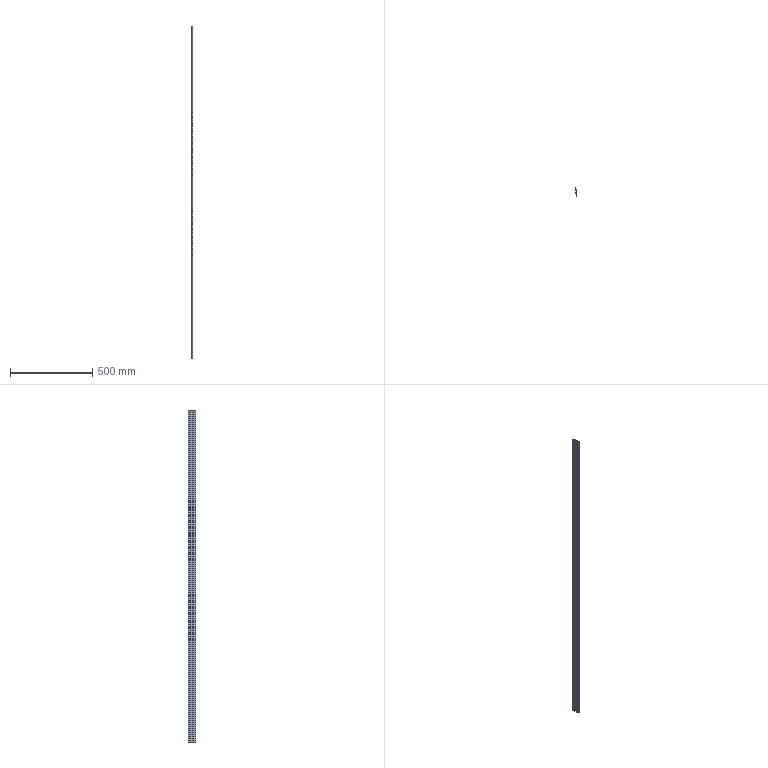Part | 1 solid | 33 faces | box 9.4 x 46.998 x 2016 mm | volume 227729 mm3 | plane 22 | cylinder 11 | commonest cylinder face diameters 0.24 x2 0.4 x2 0.8 x2 1.2 x2 6 x2 1 x1
STEP:
#1=CARTESIAN_POINT('',(-2.9,32.45,-1008.));
#2=VERTEX_POINT('',#1);
#3=CARTESIAN_POINT('',(-2.7,32.25,-1008.));
#4=VERTEX_POINT('',#3);
#5=CARTESIAN_POINT('',(-2.7,32.45,-1008.));
#6=DIRECTION('',(0.,0.,1.));
#7=DIRECTION('',(1.,0.,0.));
#8=AXIS2_PLACEMENT_3D('',#5,#6,#7);
#9=CIRCLE('',#8,0.2);
#10=EDGE_CURVE('',#2,#4,#9,.T.);
#11=ORIENTED_EDGE('',*,*,#10,.T.);
#12=CARTESIAN_POINT('',(-2.7,32.25,1008.));
#13=VERTEX_POINT('',#12);
#14=CARTESIAN_POINT('',(-2.7,32.25,1008.));
#15=DIRECTION('',(0.,0.,-1.));
#16=VECTOR('',#15,1000.);
#17=LINE('',#14,#16);
#18=EDGE_CURVE('',#13,#4,#17,.T.);
#19=ORIENTED_EDGE('',*,*,#18,.F.);
#20=CARTESIAN_POINT('',(-2.9,32.45,1008.));
#21=VERTEX_POINT('',#20);
#22=CARTESIAN_POINT('',(-2.7,32.45,1008.));
#23=DIRECTION('',(0.,0.,1.));
#24=DIRECTION('',(1.,0.,0.));
#25=AXIS2_PLACEMENT_3D('',#22,#23,#24);
#26=CIRCLE('',#25,0.2);
#27=EDGE_CURVE('',#21,#13,#26,.T.);
#28=ORIENTED_EDGE('',*,*,#27,.F.);
#29=CARTESIAN_POINT('',(-2.9,32.45,1008.));
#30=DIRECTION('',(0.,0.,-1.));
#31=VECTOR('',#30,1000.);
#32=LINE('',#29,#31);
#33=EDGE_CURVE('',#21,#2,#32,.T.);
#34=ORIENTED_EDGE('',*,*,#33,.T.);
#35=EDGE_LOOP('',(#11,#19,#28,#34));
#36=FACE_OUTER_BOUND('',#35,.T.);
#37=CARTESIAN_POINT('',(-2.7,32.45,1008.));
#38=DIRECTION('',(0.,0.,-1.));
#39=DIRECTION('',(-1.,0.,0.));
#40=AXIS2_PLACEMENT_3D('',#37,#38,#39);
#41=CYLINDRICAL_SURFACE('',#40,0.2);
#42=ADVANCED_FACE('',(#36),#41,.T.);
#43=CARTESIAN_POINT('',(-2.5,32.25,-1008.));
#44=VERTEX_POINT('',#43);
#45=CARTESIAN_POINT('',(-2.7,32.25,-1008.));
#46=DIRECTION('',(1.,0.,0.));
#47=VECTOR('',#46,1000.);
#48=LINE('',#45,#47);
#49=EDGE_CURVE('',#4,#44,#48,.T.);
#50=ORIENTED_EDGE('',*,*,#49,.T.);
#51=CARTESIAN_POINT('',(-2.5,32.25,1008.));
#52=VERTEX_POINT('',#51);
#53=CARTESIAN_POINT('',(-2.5,32.25,1008.));
#54=DIRECTION('',(0.,0.,-1.));
#55=VECTOR('',#54,1000.);
#56=LINE('',#53,#55);
#57=EDGE_CURVE('',#52,#44,#56,.T.);
#58=ORIENTED_EDGE('',*,*,#57,.F.);
#59=CARTESIAN_POINT('',(-2.7,32.25,1008.));
#60=DIRECTION('',(1.,0.,0.));
#61=VECTOR('',#60,1000.);
#62=LINE('',#59,#61);
#63=EDGE_CURVE('',#13,#52,#62,.T.);
#64=ORIENTED_EDGE('',*,*,#63,.F.);
#65=ORIENTED_EDGE('',*,*,#18,.T.);
#66=EDGE_LOOP('',(#50,#58,#64,#65));
#67=FACE_OUTER_BOUND('',#66,.T.);
#68=CARTESIAN_POINT('',(-2.7,32.25,1008.));
#69=DIRECTION('',(0.,1.,0.));
#70=DIRECTION('',(0.,0.,1.));
#71=AXIS2_PLACEMENT_3D('',#68,#69,#70);
#72=PLANE('',#71);
#73=ADVANCED_FACE('',(#67),#72,.F.);
#74=CARTESIAN_POINT('',(-1.9,32.85,-1008.));
#75=VERTEX_POINT('',#74);
#76=CARTESIAN_POINT('',(-2.5,32.85,-1008.));
#77=DIRECTION('',(0.,0.,1.));
#78=DIRECTION('',(1.,0.,0.));
#79=AXIS2_PLACEMENT_3D('',#76,#77,#78);
#80=CIRCLE('',#79,0.6);
#81=EDGE_CURVE('',#44,#75,#80,.T.);
#82=ORIENTED_EDGE('',*,*,#81,.T.);
#83=CARTESIAN_POINT('',(-1.9,32.85,1008.));
#84=VERTEX_POINT('',#83);
#85=CARTESIAN_POINT('',(-1.9,32.85,1008.));
#86=DIRECTION('',(0.,0.,-1.));
#87=VECTOR('',#86,1000.);
#88=LINE('',#85,#87);
#89=EDGE_CURVE('',#84,#75,#88,.T.);
#90=ORIENTED_EDGE('',*,*,#89,.F.);
#91=CARTESIAN_POINT('',(-2.5,32.85,1008.));
#92=DIRECTION('',(0.,0.,1.));
#93=DIRECTION('',(1.,0.,0.));
#94=AXIS2_PLACEMENT_3D('',#91,#92,#93);
#95=CIRCLE('',#94,0.6);
#96=EDGE_CURVE('',#52,#84,#95,.T.);
#97=ORIENTED_EDGE('',*,*,#96,.F.);
#98=ORIENTED_EDGE('',*,*,#57,.T.);
#99=EDGE_LOOP('',(#82,#90,#97,#98));
#100=FACE_OUTER_BOUND('',#99,.T.);
#101=CARTESIAN_POINT('',(-2.5,32.85,1008.));
#102=DIRECTION('',(0.,0.,-1.));
#103=DIRECTION('',(-1.,0.,0.));
#104=AXIS2_PLACEMENT_3D('',#101,#102,#103);
#105=CYLINDRICAL_SURFACE('',#104,0.6);
#106=ADVANCED_FACE('',(#100),#105,.T.);
#107=CARTESIAN_POINT('',(-1.9,36.13,-1008.));
#108=VERTEX_POINT('',#107);
#109=CARTESIAN_POINT('',(-1.9,32.85,-1008.));
#110=DIRECTION('',(0.,1.,0.));
#111=VECTOR('',#110,1000.);
#112=LINE('',#109,#111);
#113=EDGE_CURVE('',#75,#108,#112,.T.);
#114=ORIENTED_EDGE('',*,*,#113,.T.);
#115=CARTESIAN_POINT('',(-1.9,36.13,1008.));
#116=VERTEX_POINT('',#115);
#117=CARTESIAN_POINT('',(-1.9,36.13,1008.));
#118=DIRECTION('',(0.,0.,-1.));
#119=VECTOR('',#118,1000.);
#120=LINE('',#117,#119);
#121=EDGE_CURVE('',#116,#108,#120,.T.);
#122=ORIENTED_EDGE('',*,*,#121,.F.);
#123=CARTESIAN_POINT('',(-1.9,32.85,1008.));
#124=DIRECTION('',(0.,1.,0.));
#125=VECTOR('',#124,1000.);
#126=LINE('',#123,#125);
#127=EDGE_CURVE('',#84,#116,#126,.T.);
#128=ORIENTED_EDGE('',*,*,#127,.F.);
#129=ORIENTED_EDGE('',*,*,#89,.T.);
#130=EDGE_LOOP('',(#114,#122,#128,#129));
#131=FACE_OUTER_BOUND('',#130,.T.);
#132=CARTESIAN_POINT('',(-1.9,32.85,1008.));
#133=DIRECTION('',(-1.,0.,0.));
#134=DIRECTION('',(0.,0.,1.));
#135=AXIS2_PLACEMENT_3D('',#132,#133,#134);
#136=PLANE('',#135);
#137=ADVANCED_FACE('',(#131),#136,.F.);
#138=CARTESIAN_POINT('',(-1.78,36.25,-1008.));
#139=VERTEX_POINT('',#138);
#140=CARTESIAN_POINT('',(-1.78,36.13,-1008.));
#141=DIRECTION('',(0.,0.,-1.));
#142=DIRECTION('',(1.,0.,0.));
#143=AXIS2_PLACEMENT_3D('',#140,#141,#142);
#144=CIRCLE('',#143,0.12);
#145=EDGE_CURVE('',#108,#139,#144,.T.);
#146=ORIENTED_EDGE('',*,*,#145,.T.);
#147=CARTESIAN_POINT('',(-1.78,36.25,1008.));
#148=VERTEX_POINT('',#147);
#149=CARTESIAN_POINT('',(-1.78,36.25,1008.));
#150=DIRECTION('',(0.,0.,-1.));
#151=VECTOR('',#150,1000.);
#152=LINE('',#149,#151);
#153=EDGE_CURVE('',#148,#139,#152,.T.);
#154=ORIENTED_EDGE('',*,*,#153,.F.);
#155=CARTESIAN_POINT('',(-1.78,36.13,1008.));
#156=DIRECTION('',(0.,0.,-1.));
#157=DIRECTION('',(1.,0.,0.));
#158=AXIS2_PLACEMENT_3D('',#155,#156,#157);
#159=CIRCLE('',#158,0.12);
#160=EDGE_CURVE('',#116,#148,#159,.T.);
#161=ORIENTED_EDGE('',*,*,#160,.F.);
#162=ORIENTED_EDGE('',*,*,#121,.T.);
#163=EDGE_LOOP('',(#146,#154,#161,#162));
#164=FACE_OUTER_BOUND('',#163,.T.);
#165=CARTESIAN_POINT('',(-1.78,36.13,1008.));
#166=DIRECTION('',(0.,0.,-1.));
#167=DIRECTION('',(-1.,0.,0.));
#168=AXIS2_PLACEMENT_3D('',#165,#166,#167);
#169=CYLINDRICAL_SURFACE('',#168,0.12);
#170=ADVANCED_FACE('',(#164),#169,.F.);
#171=CARTESIAN_POINT('',(0.,36.25,-1008.));
#172=VERTEX_POINT('',#171);
#173=CARTESIAN_POINT('',(-1.78,36.25,-1008.));
#174=DIRECTION('',(1.,0.,0.));
#175=VECTOR('',#174,1000.);
#176=LINE('',#173,#175);
#177=EDGE_CURVE('',#139,#172,#176,.T.);
#178=ORIENTED_EDGE('',*,*,#177,.T.);
#179=CARTESIAN_POINT('',(0.,36.25,1008.));
#180=VERTEX_POINT('',#179);
#181=CARTESIAN_POINT('',(0.,36.25,1008.));
#182=DIRECTION('',(0.,0.,-1.));
#183=VECTOR('',#182,1000.);
#184=LINE('',#181,#183);
#185=EDGE_CURVE('',#180,#172,#184,.T.);
#186=ORIENTED_EDGE('',*,*,#185,.F.);
#187=CARTESIAN_POINT('',(-1.78,36.25,1008.));
#188=DIRECTION('',(1.,0.,0.));
#189=VECTOR('',#188,1000.);
#190=LINE('',#187,#189);
#191=EDGE_CURVE('',#148,#180,#190,.T.);
#192=ORIENTED_EDGE('',*,*,#191,.F.);
#193=ORIENTED_EDGE('',*,*,#153,.T.);
#194=EDGE_LOOP('',(#178,#186,#192,#193));
#195=FACE_OUTER_BOUND('',#194,.T.);
#196=CARTESIAN_POINT('',(-1.78,36.25,1008.));
#197=DIRECTION('',(0.,1.,0.));
#198=DIRECTION('',(0.,0.,1.));
#199=AXIS2_PLACEMENT_3D('',#196,#197,#198);
#200=PLANE('',#199);
#201=ADVANCED_FACE('',(#195),#200,.F.);
#202=CARTESIAN_POINT('',(0.0007641,20.449,-1008.));
#203=VERTEX_POINT('',#202);
#204=CARTESIAN_POINT('',(0.,36.25,-1008.));
#205=DIRECTION('',(0.00004836,-1.,0.));
#206=VECTOR('',#205,1000.);
#207=LINE('',#204,#206);
#208=EDGE_CURVE('',#172,#203,#207,.T.);
#209=ORIENTED_EDGE('',*,*,#208,.T.);
#210=CARTESIAN_POINT('',(0.0007641,20.449,1008.));
#211=VERTEX_POINT('',#210);
#212=CARTESIAN_POINT('',(0.0007641,20.449,1008.));
#213=DIRECTION('',(0.,0.,-1.));
#214=VECTOR('',#213,1000.);
#215=LINE('',#212,#214);
#216=EDGE_CURVE('',#211,#203,#215,.T.);
#217=ORIENTED_EDGE('',*,*,#216,.F.);
#218=CARTESIAN_POINT('',(0.,36.25,1008.));
#219=DIRECTION('',(0.00004836,-1.,0.));
#220=VECTOR('',#219,1000.);
#221=LINE('',#218,#220);
#222=EDGE_CURVE('',#180,#211,#221,.T.);
#223=ORIENTED_EDGE('',*,*,#222,.F.);
#224=ORIENTED_EDGE('',*,*,#185,.T.);
#225=EDGE_LOOP('',(#209,#217,#223,#224));
#226=FACE_OUTER_BOUND('',#225,.T.);
#227=CARTESIAN_POINT('',(0.,36.25,1008.));
#228=DIRECTION('',(1.,0.00004836,0.));
#229=DIRECTION('',(-0.00004836,1.,0.));
#230=AXIS2_PLACEMENT_3D('',#227,#228,#229);
#231=PLANE('',#230);
#232=ADVANCED_FACE('',(#226),#231,.F.);
#233=CARTESIAN_POINT('',(-2.499,20.449,-1008.));
#234=VERTEX_POINT('',#233);
#235=CARTESIAN_POINT('',(0.0007641,20.449,-1008.));
#236=DIRECTION('',(-1.,0.,0.));
#237=VECTOR('',#236,1000.);
#238=LINE('',#235,#237);
#239=EDGE_CURVE('',#203,#234,#238,.T.);
#240=ORIENTED_EDGE('',*,*,#239,.T.);
#241=CARTESIAN_POINT('',(-2.499,20.449,1008.));
#242=VERTEX_POINT('',#241);
#243=CARTESIAN_POINT('',(-2.499,20.449,1008.));
#244=DIRECTION('',(0.,0.,-1.));
#245=VECTOR('',#244,1000.);
#246=LINE('',#243,#245);
#247=EDGE_CURVE('',#242,#234,#246,.T.);
#248=ORIENTED_EDGE('',*,*,#247,.F.);
#249=CARTESIAN_POINT('',(0.0007641,20.449,1008.));
#250=DIRECTION('',(-1.,0.,0.));
#251=VECTOR('',#250,1000.);
#252=LINE('',#249,#251);
#253=EDGE_CURVE('',#211,#242,#252,.T.);
#254=ORIENTED_EDGE('',*,*,#253,.F.);
#255=ORIENTED_EDGE('',*,*,#216,.T.);
#256=EDGE_LOOP('',(#240,#248,#254,#255));
#257=FACE_OUTER_BOUND('',#256,.T.);
#258=CARTESIAN_POINT('',(0.0007641,20.449,1008.));
#259=DIRECTION('',(0.,-1.,0.));
#260=DIRECTION('',(0.,0.,-1.));
#261=AXIS2_PLACEMENT_3D('',#258,#259,#260);
#262=PLANE('',#261);
#263=ADVANCED_FACE('',(#257),#262,.F.);
#264=CARTESIAN_POINT('',(-2.899,20.049,-1008.));
#265=VERTEX_POINT('',#264);
#266=CARTESIAN_POINT('',(-2.499,20.049,-1008.));
#267=DIRECTION('',(0.,0.,1.));
#268=DIRECTION('',(1.,0.,0.));
#269=AXIS2_PLACEMENT_3D('',#266,#267,#268);
#270=CIRCLE('',#269,0.4);
#271=EDGE_CURVE('',#234,#265,#270,.T.);
#272=ORIENTED_EDGE('',*,*,#271,.T.);
#273=CARTESIAN_POINT('',(-2.899,20.049,1008.));
#274=VERTEX_POINT('',#273);
#275=CARTESIAN_POINT('',(-2.899,20.049,1008.));
#276=DIRECTION('',(0.,0.,-1.));
#277=VECTOR('',#276,1000.);
#278=LINE('',#275,#277);
#279=EDGE_CURVE('',#274,#265,#278,.T.);
#280=ORIENTED_EDGE('',*,*,#279,.F.);
#281=CARTESIAN_POINT('',(-2.499,20.049,1008.));
#282=DIRECTION('',(0.,0.,1.));
#283=DIRECTION('',(1.,0.,0.));
#284=AXIS2_PLACEMENT_3D('',#281,#282,#283);
#285=CIRCLE('',#284,0.4);
#286=EDGE_CURVE('',#242,#274,#285,.T.);
#287=ORIENTED_EDGE('',*,*,#286,.F.);
#288=ORIENTED_EDGE('',*,*,#247,.T.);
#289=EDGE_LOOP('',(#272,#280,#287,#288));
#290=FACE_OUTER_BOUND('',#289,.T.);
#291=CARTESIAN_POINT('',(-2.499,20.049,1008.));
#292=DIRECTION('',(0.,0.,-1.));
#293=DIRECTION('',(-1.,0.,0.));
#294=AXIS2_PLACEMENT_3D('',#291,#292,#293);
#295=CYLINDRICAL_SURFACE('',#294,0.4);
#296=ADVANCED_FACE('',(#290),#295,.T.);
#297=CARTESIAN_POINT('',(-2.899,15.65,-1008.));
#298=VERTEX_POINT('',#297);
#299=CARTESIAN_POINT('',(-2.899,20.049,-1008.));
#300=DIRECTION('',(0.,-1.,0.));
#301=VECTOR('',#300,1000.);
#302=LINE('',#299,#301);
#303=EDGE_CURVE('',#265,#298,#302,.T.);
#304=ORIENTED_EDGE('',*,*,#303,.T.);
#305=CARTESIAN_POINT('',(-2.899,15.65,1008.));
#306=VERTEX_POINT('',#305);
#307=CARTESIAN_POINT('',(-2.899,15.65,1008.));
#308=DIRECTION('',(0.,0.,-1.));
#309=VECTOR('',#308,1000.);
#310=LINE('',#307,#309);
#311=EDGE_CURVE('',#306,#298,#310,.T.);
#312=ORIENTED_EDGE('',*,*,#311,.F.);
#313=CARTESIAN_POINT('',(-2.899,20.049,1008.));
#314=DIRECTION('',(0.,-1.,0.));
#315=VECTOR('',#314,1000.);
#316=LINE('',#313,#315);
#317=EDGE_CURVE('',#274,#306,#316,.T.);
#318=ORIENTED_EDGE('',*,*,#317,.F.);
#319=ORIENTED_EDGE('',*,*,#279,.T.);
#320=EDGE_LOOP('',(#304,#312,#318,#319));
#321=FACE_OUTER_BOUND('',#320,.T.);
#322=CARTESIAN_POINT('',(-2.899,20.049,1008.));
#323=DIRECTION('',(1.,0.,0.));
#324=DIRECTION('',(0.,0.,-1.));
#325=AXIS2_PLACEMENT_3D('',#322,#323,#324);
#326=PLANE('',#325);
#327=ADVANCED_FACE('',(#321),#326,.F.);
#328=CARTESIAN_POINT('',(-2.699,15.45,-1008.));
#329=VERTEX_POINT('',#328);
#330=CARTESIAN_POINT('',(-2.699,15.65,-1008.));
#331=DIRECTION('',(0.,0.,1.));
#332=DIRECTION('',(1.,0.,0.));
#333=AXIS2_PLACEMENT_3D('',#330,#331,#332);
#334=CIRCLE('',#333,0.2);
#335=EDGE_CURVE('',#298,#329,#334,.T.);
#336=ORIENTED_EDGE('',*,*,#335,.T.);
#337=CARTESIAN_POINT('',(-2.699,15.45,1008.));
#338=VERTEX_POINT('',#337);
#339=CARTESIAN_POINT('',(-2.699,15.45,1008.));
#340=DIRECTION('',(0.,0.,-1.));
#341=VECTOR('',#340,1000.);
#342=LINE('',#339,#341);
#343=EDGE_CURVE('',#338,#329,#342,.T.);
#344=ORIENTED_EDGE('',*,*,#343,.F.);
#345=CARTESIAN_POINT('',(-2.699,15.65,1008.));
#346=DIRECTION('',(0.,0.,1.));
#347=DIRECTION('',(1.,0.,0.));
#348=AXIS2_PLACEMENT_3D('',#345,#346,#347);
#349=CIRCLE('',#348,0.2);
#350=EDGE_CURVE('',#306,#338,#349,.T.);
#351=ORIENTED_EDGE('',*,*,#350,.F.);
#352=ORIENTED_EDGE('',*,*,#311,.T.);
#353=EDGE_LOOP('',(#336,#344,#351,#352));
#354=FACE_OUTER_BOUND('',#353,.T.);
#355=CARTESIAN_POINT('',(-2.699,15.65,1008.));
#356=DIRECTION('',(0.,0.,-1.));
#357=DIRECTION('',(-1.,0.,0.));
#358=AXIS2_PLACEMENT_3D('',#355,#356,#357);
#359=CYLINDRICAL_SURFACE('',#358,0.2);
#360=ADVANCED_FACE('',(#354),#359,.T.);
#361=CARTESIAN_POINT('',(-2.499,15.45,-1008.));
#362=VERTEX_POINT('',#361);
#363=CARTESIAN_POINT('',(-2.699,15.45,-1008.));
#364=DIRECTION('',(1.,0.,0.));
#365=VECTOR('',#364,1000.);
#366=LINE('',#363,#365);
#367=EDGE_CURVE('',#329,#362,#366,.T.);
#368=ORIENTED_EDGE('',*,*,#367,.T.);
#369=CARTESIAN_POINT('',(-2.499,15.45,1008.));
#370=VERTEX_POINT('',#369);
#371=CARTESIAN_POINT('',(-2.499,15.45,1008.));
#372=DIRECTION('',(0.,0.,-1.));
#373=VECTOR('',#372,1000.);
#374=LINE('',#371,#373);
#375=EDGE_CURVE('',#370,#362,#374,.T.);
#376=ORIENTED_EDGE('',*,*,#375,.F.);
#377=CARTESIAN_POINT('',(-2.699,15.45,1008.));
#378=DIRECTION('',(1.,0.,0.));
#379=VECTOR('',#378,1000.);
#380=LINE('',#377,#379);
#381=EDGE_CURVE('',#338,#370,#380,.T.);
#382=ORIENTED_EDGE('',*,*,#381,.F.);
#383=ORIENTED_EDGE('',*,*,#343,.T.);
#384=EDGE_LOOP('',(#368,#376,#382,#383));
#385=FACE_OUTER_BOUND('',#384,.T.);
#386=CARTESIAN_POINT('',(-2.699,15.45,1008.));
#387=DIRECTION('',(0.,1.,0.));
#388=DIRECTION('',(0.,0.,1.));
#389=AXIS2_PLACEMENT_3D('',#386,#387,#388);
#390=PLANE('',#389);
#391=ADVANCED_FACE('',(#385),#390,.F.);
#392=CARTESIAN_POINT('',(-1.899,16.05,-1008.));
#393=VERTEX_POINT('',#392);
#394=CARTESIAN_POINT('',(-2.499,16.05,-1008.));
#395=DIRECTION('',(0.,0.,1.));
#396=DIRECTION('',(1.,0.,0.));
#397=AXIS2_PLACEMENT_3D('',#394,#395,#396);
#398=CIRCLE('',#397,0.6);
#399=EDGE_CURVE('',#362,#393,#398,.T.);
#400=ORIENTED_EDGE('',*,*,#399,.T.);
#401=CARTESIAN_POINT('',(-1.899,16.05,1008.));
#402=VERTEX_POINT('',#401);
#403=CARTESIAN_POINT('',(-1.899,16.05,1008.));
#404=DIRECTION('',(0.,0.,-1.));
#405=VECTOR('',#404,1000.);
#406=LINE('',#403,#405);
#407=EDGE_CURVE('',#402,#393,#406,.T.);
#408=ORIENTED_EDGE('',*,*,#407,.F.);
#409=CARTESIAN_POINT('',(-2.499,16.05,1008.));
#410=DIRECTION('',(0.,0.,1.));
#411=DIRECTION('',(1.,0.,0.));
#412=AXIS2_PLACEMENT_3D('',#409,#410,#411);
#413=CIRCLE('',#412,0.6);
#414=EDGE_CURVE('',#370,#402,#413,.T.);
#415=ORIENTED_EDGE('',*,*,#414,.F.);
#416=ORIENTED_EDGE('',*,*,#375,.T.);
#417=EDGE_LOOP('',(#400,#408,#415,#416));
#418=FACE_OUTER_BOUND('',#417,.T.);
#419=CARTESIAN_POINT('',(-2.499,16.05,1008.));
#420=DIRECTION('',(0.,0.,-1.));
#421=DIRECTION('',(-1.,0.,0.));
#422=AXIS2_PLACEMENT_3D('',#419,#420,#421);
#423=CYLINDRICAL_SURFACE('',#422,0.6);
#424=ADVANCED_FACE('',(#418),#423,.T.);
#425=CARTESIAN_POINT('',(-1.899,19.329,-1008.));
#426=VERTEX_POINT('',#425);
#427=CARTESIAN_POINT('',(-1.899,16.05,-1008.));
#428=DIRECTION('',(0.,1.,0.));
#429=VECTOR('',#428,1000.);
#430=LINE('',#427,#429);
#431=EDGE_CURVE('',#393,#426,#430,.T.);
#432=ORIENTED_EDGE('',*,*,#431,.T.);
#433=CARTESIAN_POINT('',(-1.899,19.329,1008.));
#434=VERTEX_POINT('',#433);
#435=CARTESIAN_POINT('',(-1.899,19.329,1008.));
#436=DIRECTION('',(0.,0.,-1.));
#437=VECTOR('',#436,1000.);
#438=LINE('',#435,#437);
#439=EDGE_CURVE('',#434,#426,#438,.T.);
#440=ORIENTED_EDGE('',*,*,#439,.F.);
#441=CARTESIAN_POINT('',(-1.899,16.05,1008.));
#442=DIRECTION('',(0.,1.,0.));
#443=VECTOR('',#442,1000.);
#444=LINE('',#441,#443);
#445=EDGE_CURVE('',#402,#434,#444,.T.);
#446=ORIENTED_EDGE('',*,*,#445,.F.);
#447=ORIENTED_EDGE('',*,*,#407,.T.);
#448=EDGE_LOOP('',(#432,#440,#446,#447));
#449=FACE_OUTER_BOUND('',#448,.T.);
#450=CARTESIAN_POINT('',(-1.899,16.05,1008.));
#451=DIRECTION('',(-1.,0.,0.));
#452=DIRECTION('',(0.,0.,1.));
#453=AXIS2_PLACEMENT_3D('',#450,#451,#452);
#454=PLANE('',#453);
#455=ADVANCED_FACE('',(#449),#454,.F.);
#456=CARTESIAN_POINT('',(-1.779,19.449,-1008.));
#457=VERTEX_POINT('',#456);
#458=CARTESIAN_POINT('',(-1.779,19.329,-1008.));
#459=DIRECTION('',(0.,0.,-1.));
#460=DIRECTION('',(1.,0.,0.));
#461=AXIS2_PLACEMENT_3D('',#458,#459,#460);
#462=CIRCLE('',#461,0.12);
#463=EDGE_CURVE('',#426,#457,#462,.T.);
#464=ORIENTED_EDGE('',*,*,#463,.T.);
#465=CARTESIAN_POINT('',(-1.779,19.449,1008.));
#466=VERTEX_POINT('',#465);
#467=CARTESIAN_POINT('',(-1.779,19.449,1008.));
#468=DIRECTION('',(0.,0.,-1.));
#469=VECTOR('',#468,1000.);
#470=LINE('',#467,#469);
#471=EDGE_CURVE('',#466,#457,#470,.T.);
#472=ORIENTED_EDGE('',*,*,#471,.F.);
#473=CARTESIAN_POINT('',(-1.779,19.329,1008.));
#474=DIRECTION('',(0.,0.,-1.));
#475=DIRECTION('',(1.,0.,0.));
#476=AXIS2_PLACEMENT_3D('',#473,#474,#475);
#477=CIRCLE('',#476,0.12);
#478=EDGE_CURVE('',#434,#466,#477,.T.);
#479=ORIENTED_EDGE('',*,*,#478,.F.);
#480=ORIENTED_EDGE('',*,*,#439,.T.);
#481=EDGE_LOOP('',(#464,#472,#479,#480));
#482=FACE_OUTER_BOUND('',#481,.T.);
#483=CARTESIAN_POINT('',(-1.779,19.329,1008.));
#484=DIRECTION('',(0.,0.,-1.));
#485=DIRECTION('',(-1.,0.,0.));
#486=AXIS2_PLACEMENT_3D('',#483,#484,#485);
#487=CYLINDRICAL_SURFACE('',#486,0.12);
#488=ADVANCED_FACE('',(#482),#487,.F.);
#489=CARTESIAN_POINT('',(0.0007641,19.449,-1008.));
#490=VERTEX_POINT('',#489);
#491=CARTESIAN_POINT('',(-1.779,19.449,-1008.));
#492=DIRECTION('',(1.,0.,0.));
#493=VECTOR('',#492,1000.);
#494=LINE('',#491,#493);
#495=EDGE_CURVE('',#457,#490,#494,.T.);
#496=ORIENTED_EDGE('',*,*,#495,.T.);
#497=CARTESIAN_POINT('',(0.0007641,19.449,1008.));
#498=VERTEX_POINT('',#497);
#499=CARTESIAN_POINT('',(0.0007641,19.449,1008.));
#500=DIRECTION('',(0.,0.,-1.));
#501=VECTOR('',#500,1000.);
#502=LINE('',#499,#501);
#503=EDGE_CURVE('',#498,#490,#502,.T.);
#504=ORIENTED_EDGE('',*,*,#503,.F.);
#505=CARTESIAN_POINT('',(-1.779,19.449,1008.));
#506=DIRECTION('',(1.,0.,0.));
#507=VECTOR('',#506,1000.);
#508=LINE('',#505,#507);
#509=EDGE_CURVE('',#466,#498,#508,.T.);
#510=ORIENTED_EDGE('',*,*,#509,.F.);
#511=ORIENTED_EDGE('',*,*,#471,.T.);
#512=EDGE_LOOP('',(#496,#504,#510,#511));
#513=FACE_OUTER_BOUND('',#512,.T.);
#514=CARTESIAN_POINT('',(-1.779,19.449,1008.));
#515=DIRECTION('',(0.,1.,0.));
#516=DIRECTION('',(0.,0.,1.));
#517=AXIS2_PLACEMENT_3D('',#514,#515,#516);
#518=PLANE('',#517);
#519=ADVANCED_FACE('',(#513),#518,.F.);
#520=CARTESIAN_POINT('',(0.,0.,-1008.));
#521=VERTEX_POINT('',#520);
#522=CARTESIAN_POINT('',(0.0007641,19.449,-1008.));
#523=DIRECTION('',(-0.00003929,-1.,0.));
#524=VECTOR('',#523,1000.);
#525=LINE('',#522,#524);
#526=EDGE_CURVE('',#490,#521,#525,.T.);
#527=ORIENTED_EDGE('',*,*,#526,.T.);
#528=CARTESIAN_POINT('',(0.,0.,1008.));
#529=VERTEX_POINT('',#528);
#530=CARTESIAN_POINT('',(0.,0.,1008.));
#531=DIRECTION('',(0.,0.,-1.));
#532=VECTOR('',#531,1000.);
#533=LINE('',#530,#532);
#534=EDGE_CURVE('',#529,#521,#533,.T.);
#535=ORIENTED_EDGE('',*,*,#534,.F.);
#536=CARTESIAN_POINT('',(0.0007641,19.449,1008.));
#537=DIRECTION('',(-0.00003929,-1.,0.));
#538=VECTOR('',#537,1000.);
#539=LINE('',#536,#538);
#540=EDGE_CURVE('',#498,#529,#539,.T.);
#541=ORIENTED_EDGE('',*,*,#540,.F.);
#542=ORIENTED_EDGE('',*,*,#503,.T.);
#543=EDGE_LOOP('',(#527,#535,#541,#542));
#544=FACE_OUTER_BOUND('',#543,.T.);
#545=CARTESIAN_POINT('',(0.0007641,19.449,1008.));
#546=DIRECTION('',(1.,-0.00003929,0.));
#547=DIRECTION('',(0.00003929,1.,0.));
#548=AXIS2_PLACEMENT_3D('',#545,#546,#547);
#549=PLANE('',#548);
#550=ADVANCED_FACE('',(#544),#549,.F.);
#551=CARTESIAN_POINT('',(1.5,0.,-1008.));
#552=VERTEX_POINT('',#551);
#553=CARTESIAN_POINT('',(0.,0.,-1008.));
#554=DIRECTION('',(1.,0.,0.));
#555=VECTOR('',#554,1000.);
#556=LINE('',#553,#555);
#557=EDGE_CURVE('',#521,#552,#556,.T.);
#558=ORIENTED_EDGE('',*,*,#557,.T.);
#559=CARTESIAN_POINT('',(1.5,0.,1008.));
#560=VERTEX_POINT('',#559);
#561=CARTESIAN_POINT('',(1.5,0.,1008.));
#562=DIRECTION('',(0.,0.,-1.));
#563=VECTOR('',#562,1000.);
#564=LINE('',#561,#563);
#565=EDGE_CURVE('',#560,#552,#564,.T.);
#566=ORIENTED_EDGE('',*,*,#565,.F.);
#567=CARTESIAN_POINT('',(0.,0.,1008.));
#568=DIRECTION('',(1.,0.,0.));
#569=VECTOR('',#568,1000.);
#570=LINE('',#567,#569);
#571=EDGE_CURVE('',#529,#560,#570,.T.);
#572=ORIENTED_EDGE('',*,*,#571,.F.);
#573=ORIENTED_EDGE('',*,*,#534,.T.);
#574=EDGE_LOOP('',(#558,#566,#572,#573));
#575=FACE_OUTER_BOUND('',#574,.T.);
#576=CARTESIAN_POINT('',(0.,0.,1008.));
#577=DIRECTION('',(0.,1.,0.));
#578=DIRECTION('',(0.,0.,1.));
#579=AXIS2_PLACEMENT_3D('',#576,#577,#578);
#580=PLANE('',#579);
#581=ADVANCED_FACE('',(#575),#580,.F.);
#582=CARTESIAN_POINT('',(2.,0.5,-1008.));
#583=VERTEX_POINT('',#582);
#584=CARTESIAN_POINT('',(1.5,0.5,-1008.));
#585=DIRECTION('',(0.,0.,1.));
#586=DIRECTION('',(1.,0.,0.));
#587=AXIS2_PLACEMENT_3D('',#584,#585,#586);
#588=CIRCLE('',#587,0.5);
#589=EDGE_CURVE('',#552,#583,#588,.T.);
#590=ORIENTED_EDGE('',*,*,#589,.T.);
#591=CARTESIAN_POINT('',(2.,0.5,1008.));
#592=VERTEX_POINT('',#591);
#593=CARTESIAN_POINT('',(2.,0.5,1008.));
#594=DIRECTION('',(0.,0.,-1.));
#595=VECTOR('',#594,1000.);
#596=LINE('',#593,#595);
#597=EDGE_CURVE('',#592,#583,#596,.T.);
#598=ORIENTED_EDGE('',*,*,#597,.F.);
#599=CARTESIAN_POINT('',(1.5,0.5,1008.));
#600=DIRECTION('',(0.,0.,1.));
#601=DIRECTION('',(1.,0.,0.));
#602=AXIS2_PLACEMENT_3D('',#599,#600,#601);
#603=CIRCLE('',#602,0.5);
#604=EDGE_CURVE('',#560,#592,#603,.T.);
#605=ORIENTED_EDGE('',*,*,#604,.F.);
#606=ORIENTED_EDGE('',*,*,#565,.T.);
#607=EDGE_LOOP('',(#590,#598,#605,#606));
#608=FACE_OUTER_BOUND('',#607,.T.);
#609=CARTESIAN_POINT('',(1.5,0.5,1008.));
#610=DIRECTION('',(0.,0.,-1.));
#611=DIRECTION('',(-1.,0.,0.));
#612=AXIS2_PLACEMENT_3D('',#609,#610,#611);
#613=CYLINDRICAL_SURFACE('',#612,0.5);
#614=ADVANCED_FACE('',(#608),#613,.T.);
#615=CARTESIAN_POINT('',(2.,38.058,-1008.));
#616=VERTEX_POINT('',#615);
#617=CARTESIAN_POINT('',(2.,0.5,-1008.));
#618=DIRECTION('',(0.,1.,0.));
#619=VECTOR('',#618,1000.);
#620=LINE('',#617,#619);
#621=EDGE_CURVE('',#583,#616,#620,.T.);
#622=ORIENTED_EDGE('',*,*,#621,.T.);
#623=CARTESIAN_POINT('',(2.,38.058,1008.));
#624=VERTEX_POINT('',#623);
#625=CARTESIAN_POINT('',(2.,38.058,1008.));
#626=DIRECTION('',(0.,0.,-1.));
#627=VECTOR('',#626,1000.);
#628=LINE('',#625,#627);
#629=EDGE_CURVE('',#624,#616,#628,.T.);
#630=ORIENTED_EDGE('',*,*,#629,.F.);
#631=CARTESIAN_POINT('',(2.,0.5,1008.));
#632=DIRECTION('',(0.,1.,0.));
#633=VECTOR('',#632,1000.);
#634=LINE('',#631,#633);
#635=EDGE_CURVE('',#592,#624,#634,.T.);
#636=ORIENTED_EDGE('',*,*,#635,.F.);
#637=ORIENTED_EDGE('',*,*,#597,.T.);
#638=EDGE_LOOP('',(#622,#630,#636,#637));
#639=FACE_OUTER_BOUND('',#638,.T.);
#640=CARTESIAN_POINT('',(2.,0.5,1008.));
#641=DIRECTION('',(-1.,0.,0.));
#642=DIRECTION('',(0.,0.,1.));
#643=AXIS2_PLACEMENT_3D('',#640,#641,#642);
#644=PLANE('',#643);
#645=ADVANCED_FACE('',(#639),#644,.F.);
#646=CARTESIAN_POINT('',(1.393,39.868,-1008.));
#647=VERTEX_POINT('',#646);
#648=CARTESIAN_POINT('',(-1.,38.058,-1008.));
#649=DIRECTION('',(0.,0.,1.));
#650=DIRECTION('',(1.,0.,0.));
#651=AXIS2_PLACEMENT_3D('',#648,#649,#650);
#652=CIRCLE('',#651,3.);
#653=EDGE_CURVE('',#616,#647,#652,.T.);
#654=ORIENTED_EDGE('',*,*,#653,.T.);
#655=CARTESIAN_POINT('',(1.393,39.868,1008.));
#656=VERTEX_POINT('',#655);
#657=CARTESIAN_POINT('',(1.393,39.868,1008.));
#658=DIRECTION('',(0.,0.,-1.));
#659=VECTOR('',#658,1000.);
#660=LINE('',#657,#659);
#661=EDGE_CURVE('',#656,#647,#660,.T.);
#662=ORIENTED_EDGE('',*,*,#661,.F.);
#663=CARTESIAN_POINT('',(-1.,38.058,1008.));
#664=DIRECTION('',(0.,0.,1.));
#665=DIRECTION('',(1.,0.,0.));
#666=AXIS2_PLACEMENT_3D('',#663,#664,#665);
#667=CIRCLE('',#666,3.);
#668=EDGE_CURVE('',#624,#656,#667,.T.);
#669=ORIENTED_EDGE('',*,*,#668,.F.);
#670=ORIENTED_EDGE('',*,*,#629,.T.);
#671=EDGE_LOOP('',(#654,#662,#669,#670));
#672=FACE_OUTER_BOUND('',#671,.T.);
#673=CARTESIAN_POINT('',(-1.,38.058,1008.));
#674=DIRECTION('',(0.,0.,-1.));
#675=DIRECTION('',(-1.,0.,0.));
#676=AXIS2_PLACEMENT_3D('',#673,#674,#675);
#677=CYLINDRICAL_SURFACE('',#676,3.);
#678=ADVANCED_FACE('',(#672),#677,.T.);
#679=CARTESIAN_POINT('',(-4.,46.998,-1008.));
#680=VERTEX_POINT('',#679);
#681=CARTESIAN_POINT('',(1.393,39.868,-1008.));
#682=DIRECTION('',(-0.6032,0.7976,0.));
#683=VECTOR('',#682,1000.);
#684=LINE('',#681,#683);
#685=EDGE_CURVE('',#647,#680,#684,.T.);
#686=ORIENTED_EDGE('',*,*,#685,.T.);
#687=CARTESIAN_POINT('',(-4.,46.998,1008.));
#688=VERTEX_POINT('',#687);
#689=CARTESIAN_POINT('',(-4.,46.998,1008.));
#690=DIRECTION('',(0.,0.,-1.));
#691=VECTOR('',#690,1000.);
#692=LINE('',#689,#691);
#693=EDGE_CURVE('',#688,#680,#692,.T.);
#694=ORIENTED_EDGE('',*,*,#693,.F.);
#695=CARTESIAN_POINT('',(1.393,39.868,1008.));
#696=DIRECTION('',(-0.6032,0.7976,0.));
#697=VECTOR('',#696,1000.);
#698=LINE('',#695,#697);
#699=EDGE_CURVE('',#656,#688,#698,.T.);
#700=ORIENTED_EDGE('',*,*,#699,.F.);
#701=ORIENTED_EDGE('',*,*,#661,.T.);
#702=EDGE_LOOP('',(#686,#694,#700,#701));
#703=FACE_OUTER_BOUND('',#702,.T.);
#704=CARTESIAN_POINT('',(1.393,39.868,1008.));
#705=DIRECTION('',(-0.7976,-0.6032,0.));
#706=DIRECTION('',(0.6032,-0.7976,0.));
#707=AXIS2_PLACEMENT_3D('',#704,#705,#706);
#708=PLANE('',#707);
#709=ADVANCED_FACE('',(#703),#708,.F.);
#710=CARTESIAN_POINT('',(-7.4,46.998,-1008.));
#711=VERTEX_POINT('',#710);
#712=CARTESIAN_POINT('',(-4.,46.998,-1008.));
#713=DIRECTION('',(-1.,0.,0.));
#714=VECTOR('',#713,1000.);
#715=LINE('',#712,#714);
#716=EDGE_CURVE('',#680,#711,#715,.T.);
#717=ORIENTED_EDGE('',*,*,#716,.T.);
#718=CARTESIAN_POINT('',(-7.4,46.998,1008.));
#719=VERTEX_POINT('',#718);
#720=CARTESIAN_POINT('',(-7.4,46.998,1008.));
#721=DIRECTION('',(0.,0.,-1.));
#722=VECTOR('',#721,1000.);
#723=LINE('',#720,#722);
#724=EDGE_CURVE('',#719,#711,#723,.T.);
#725=ORIENTED_EDGE('',*,*,#724,.F.);
#726=CARTESIAN_POINT('',(-4.,46.998,1008.));
#727=DIRECTION('',(-1.,0.,0.));
#728=VECTOR('',#727,1000.);
#729=LINE('',#726,#728);
#730=EDGE_CURVE('',#688,#719,#729,.T.);
#731=ORIENTED_EDGE('',*,*,#730,.F.);
#732=ORIENTED_EDGE('',*,*,#693,.T.);
#733=EDGE_LOOP('',(#717,#725,#731,#732));
#734=FACE_OUTER_BOUND('',#733,.T.);
#735=CARTESIAN_POINT('',(-4.,46.998,1008.));
#736=DIRECTION('',(0.,-1.,0.));
#737=DIRECTION('',(0.,0.,-1.));
#738=AXIS2_PLACEMENT_3D('',#735,#736,#737);
#739=PLANE('',#738);
#740=ADVANCED_FACE('',(#734),#739,.F.);
#741=CARTESIAN_POINT('',(-7.4,45.998,-1008.));
#742=VERTEX_POINT('',#741);
#743=CARTESIAN_POINT('',(-7.4,46.998,-1008.));
#744=DIRECTION('',(0.,-1.,0.));
#745=VECTOR('',#744,1000.);
#746=LINE('',#743,#745);
#747=EDGE_CURVE('',#711,#742,#746,.T.);
#748=ORIENTED_EDGE('',*,*,#747,.T.);
#749=CARTESIAN_POINT('',(-7.4,45.998,1008.));
#750=VERTEX_POINT('',#749);
#751=CARTESIAN_POINT('',(-7.4,45.998,1008.));
#752=DIRECTION('',(0.,0.,-1.));
#753=VECTOR('',#752,1000.);
#754=LINE('',#751,#753);
#755=EDGE_CURVE('',#750,#742,#754,.T.);
#756=ORIENTED_EDGE('',*,*,#755,.F.);
#757=CARTESIAN_POINT('',(-7.4,46.998,1008.));
#758=DIRECTION('',(0.,-1.,0.));
#759=VECTOR('',#758,1000.);
#760=LINE('',#757,#759);
#761=EDGE_CURVE('',#719,#750,#760,.T.);
#762=ORIENTED_EDGE('',*,*,#761,.F.);
#763=ORIENTED_EDGE('',*,*,#724,.T.);
#764=EDGE_LOOP('',(#748,#756,#762,#763));
#765=FACE_OUTER_BOUND('',#764,.T.);
#766=CARTESIAN_POINT('',(-7.4,46.998,1008.));
#767=DIRECTION('',(1.,0.,0.));
#768=DIRECTION('',(0.,0.,-1.));
#769=AXIS2_PLACEMENT_3D('',#766,#767,#768);
#770=PLANE('',#769);
#771=ADVANCED_FACE('',(#765),#770,.F.);
#772=CARTESIAN_POINT('',(-5.751,45.998,-1008.));
#773=VERTEX_POINT('',#772);
#774=CARTESIAN_POINT('',(-7.4,45.998,-1008.));
#775=DIRECTION('',(1.,0.,0.));
#776=VECTOR('',#775,1000.);
#777=LINE('',#774,#776);
#778=EDGE_CURVE('',#742,#773,#777,.T.);
#779=ORIENTED_EDGE('',*,*,#778,.T.);
#780=CARTESIAN_POINT('',(-5.751,45.998,1008.));
#781=VERTEX_POINT('',#780);
#782=CARTESIAN_POINT('',(-5.751,45.998,1008.));
#783=DIRECTION('',(0.,0.,-1.));
#784=VECTOR('',#783,1000.);
#785=LINE('',#782,#784);
#786=EDGE_CURVE('',#781,#773,#785,.T.);
#787=ORIENTED_EDGE('',*,*,#786,.F.);
#788=CARTESIAN_POINT('',(-7.4,45.998,1008.));
#789=DIRECTION('',(1.,0.,0.));
#790=VECTOR('',#789,1000.);
#791=LINE('',#788,#790);
#792=EDGE_CURVE('',#750,#781,#791,.T.);
#793=ORIENTED_EDGE('',*,*,#792,.F.);
#794=ORIENTED_EDGE('',*,*,#755,.T.);
#795=EDGE_LOOP('',(#779,#787,#793,#794));
#796=FACE_OUTER_BOUND('',#795,.T.);
#797=CARTESIAN_POINT('',(-7.4,45.998,1008.));
#798=DIRECTION('',(0.,1.,0.));
#799=DIRECTION('',(0.,0.,1.));
#800=AXIS2_PLACEMENT_3D('',#797,#798,#799);
#801=PLANE('',#800);
#802=ADVANCED_FACE('',(#796),#801,.F.);
#803=CARTESIAN_POINT('',(-0.6072,39.196,-1008.));
#804=VERTEX_POINT('',#803);
#805=CARTESIAN_POINT('',(-5.751,45.998,-1008.));
#806=DIRECTION('',(0.6032,-0.7976,0.));
#807=VECTOR('',#806,1000.);
#808=LINE('',#805,#807);
#809=EDGE_CURVE('',#773,#804,#808,.T.);
#810=ORIENTED_EDGE('',*,*,#809,.T.);
#811=CARTESIAN_POINT('',(-0.6072,39.196,1008.));
#812=VERTEX_POINT('',#811);
#813=CARTESIAN_POINT('',(-0.6072,39.196,1008.));
#814=DIRECTION('',(0.,0.,-1.));
#815=VECTOR('',#814,1000.);
#816=LINE('',#813,#815);
#817=EDGE_CURVE('',#812,#804,#816,.T.);
#818=ORIENTED_EDGE('',*,*,#817,.F.);
#819=CARTESIAN_POINT('',(-5.751,45.998,1008.));
#820=DIRECTION('',(0.6032,-0.7976,0.));
#821=VECTOR('',#820,1000.);
#822=LINE('',#819,#821);
#823=EDGE_CURVE('',#781,#812,#822,.T.);
#824=ORIENTED_EDGE('',*,*,#823,.F.);
#825=ORIENTED_EDGE('',*,*,#786,.T.);
#826=EDGE_LOOP('',(#810,#818,#824,#825));
#827=FACE_OUTER_BOUND('',#826,.T.);
#828=CARTESIAN_POINT('',(-5.751,45.998,1008.));
#829=DIRECTION('',(0.7976,0.6032,0.));
#830=DIRECTION('',(-0.6032,0.7976,0.));
#831=AXIS2_PLACEMENT_3D('',#828,#829,#830);
#832=PLANE('',#831);
#833=ADVANCED_FACE('',(#827),#832,.F.);
#834=CARTESIAN_POINT('',(0.,37.387,-1008.));
#835=VERTEX_POINT('',#834);
#836=CARTESIAN_POINT('',(-3.,37.387,-1008.));
#837=DIRECTION('',(0.,0.,-1.));
#838=DIRECTION('',(1.,0.,0.));
#839=AXIS2_PLACEMENT_3D('',#836,#837,#838);
#840=CIRCLE('',#839,3.);
#841=EDGE_CURVE('',#804,#835,#840,.T.);
#842=ORIENTED_EDGE('',*,*,#841,.T.);
#843=CARTESIAN_POINT('',(0.,37.387,1008.));
#844=VERTEX_POINT('',#843);
#845=CARTESIAN_POINT('',(0.,37.387,1008.));
#846=DIRECTION('',(0.,0.,-1.));
#847=VECTOR('',#846,1000.);
#848=LINE('',#845,#847);
#849=EDGE_CURVE('',#844,#835,#848,.T.);
#850=ORIENTED_EDGE('',*,*,#849,.F.);
#851=CARTESIAN_POINT('',(-3.,37.387,1008.));
#852=DIRECTION('',(0.,0.,-1.));
#853=DIRECTION('',(1.,0.,0.));
#854=AXIS2_PLACEMENT_3D('',#851,#852,#853);
#855=CIRCLE('',#854,3.);
#856=EDGE_CURVE('',#812,#844,#855,.T.);
#857=ORIENTED_EDGE('',*,*,#856,.F.);
#858=ORIENTED_EDGE('',*,*,#817,.T.);
#859=EDGE_LOOP('',(#842,#850,#857,#858));
#860=FACE_OUTER_BOUND('',#859,.T.);
#861=CARTESIAN_POINT('',(-3.,37.387,1008.));
#862=DIRECTION('',(0.,0.,-1.));
#863=DIRECTION('',(-1.,0.,0.));
#864=AXIS2_PLACEMENT_3D('',#861,#862,#863);
#865=CYLINDRICAL_SURFACE('',#864,3.);
#866=ADVANCED_FACE('',(#860),#865,.F.);
#867=CARTESIAN_POINT('',(0.,37.25,-1008.));
#868=VERTEX_POINT('',#867);
#869=CARTESIAN_POINT('',(0.,37.387,-1008.));
#870=DIRECTION('',(0.,-1.,0.));
#871=VECTOR('',#870,1000.);
#872=LINE('',#869,#871);
#873=EDGE_CURVE('',#835,#868,#872,.T.);
#874=ORIENTED_EDGE('',*,*,#873,.T.);
#875=CARTESIAN_POINT('',(0.,37.25,1008.));
#876=VERTEX_POINT('',#875);
#877=CARTESIAN_POINT('',(0.,37.25,1008.));
#878=DIRECTION('',(0.,0.,-1.));
#879=VECTOR('',#878,1000.);
#880=LINE('',#877,#879);
#881=EDGE_CURVE('',#876,#868,#880,.T.);
#882=ORIENTED_EDGE('',*,*,#881,.F.);
#883=CARTESIAN_POINT('',(0.,37.387,1008.));
#884=DIRECTION('',(0.,-1.,0.));
#885=VECTOR('',#884,1000.);
#886=LINE('',#883,#885);
#887=EDGE_CURVE('',#844,#876,#886,.T.);
#888=ORIENTED_EDGE('',*,*,#887,.F.);
#889=ORIENTED_EDGE('',*,*,#849,.T.);
#890=EDGE_LOOP('',(#874,#882,#888,#889));
#891=FACE_OUTER_BOUND('',#890,.T.);
#892=CARTESIAN_POINT('',(0.,37.387,1008.));
#893=DIRECTION('',(1.,0.,0.));
#894=DIRECTION('',(0.,1.,0.));
#895=AXIS2_PLACEMENT_3D('',#892,#893,#894);
#896=PLANE('',#895);
#897=ADVANCED_FACE('',(#891),#896,.F.);
#898=CARTESIAN_POINT('',(-2.5,37.25,-1008.));
#899=VERTEX_POINT('',#898);
#900=CARTESIAN_POINT('',(0.,37.25,-1008.));
#901=DIRECTION('',(-1.,0.,0.));
#902=VECTOR('',#901,1000.);
#903=LINE('',#900,#902);
#904=EDGE_CURVE('',#868,#899,#903,.T.);
#905=ORIENTED_EDGE('',*,*,#904,.T.);
#906=CARTESIAN_POINT('',(-2.5,37.25,1008.));
#907=VERTEX_POINT('',#906);
#908=CARTESIAN_POINT('',(-2.5,37.25,1008.));
#909=DIRECTION('',(0.,0.,-1.));
#910=VECTOR('',#909,1000.);
#911=LINE('',#908,#910);
#912=EDGE_CURVE('',#907,#899,#911,.T.);
#913=ORIENTED_EDGE('',*,*,#912,.F.);
#914=CARTESIAN_POINT('',(0.,37.25,1008.));
#915=DIRECTION('',(-1.,0.,0.));
#916=VECTOR('',#915,1000.);
#917=LINE('',#914,#916);
#918=EDGE_CURVE('',#876,#907,#917,.T.);
#919=ORIENTED_EDGE('',*,*,#918,.F.);
#920=ORIENTED_EDGE('',*,*,#881,.T.);
#921=EDGE_LOOP('',(#905,#913,#919,#920));
#922=FACE_OUTER_BOUND('',#921,.T.);
#923=CARTESIAN_POINT('',(0.,37.25,1008.));
#924=DIRECTION('',(0.,-1.,0.));
#925=DIRECTION('',(0.,0.,-1.));
#926=AXIS2_PLACEMENT_3D('',#923,#924,#925);
#927=PLANE('',#926);
#928=ADVANCED_FACE('',(#922),#927,.F.);
#929=CARTESIAN_POINT('',(-2.9,36.85,-1008.));
#930=VERTEX_POINT('',#929);
#931=CARTESIAN_POINT('',(-2.5,36.85,-1008.));
#932=DIRECTION('',(0.,0.,1.));
#933=DIRECTION('',(1.,0.,0.));
#934=AXIS2_PLACEMENT_3D('',#931,#932,#933);
#935=CIRCLE('',#934,0.4);
#936=EDGE_CURVE('',#899,#930,#935,.T.);
#937=ORIENTED_EDGE('',*,*,#936,.T.);
#938=CARTESIAN_POINT('',(-2.9,36.85,1008.));
#939=VERTEX_POINT('',#938);
#940=CARTESIAN_POINT('',(-2.9,36.85,1008.));
#941=DIRECTION('',(0.,0.,-1.));
#942=VECTOR('',#941,1000.);
#943=LINE('',#940,#942);
#944=EDGE_CURVE('',#939,#930,#943,.T.);
#945=ORIENTED_EDGE('',*,*,#944,.F.);
#946=CARTESIAN_POINT('',(-2.5,36.85,1008.));
#947=DIRECTION('',(0.,0.,1.));
#948=DIRECTION('',(1.,0.,0.));
#949=AXIS2_PLACEMENT_3D('',#946,#947,#948);
#950=CIRCLE('',#949,0.4);
#951=EDGE_CURVE('',#907,#939,#950,.T.);
#952=ORIENTED_EDGE('',*,*,#951,.F.);
#953=ORIENTED_EDGE('',*,*,#912,.T.);
#954=EDGE_LOOP('',(#937,#945,#952,#953));
#955=FACE_OUTER_BOUND('',#954,.T.);
#956=CARTESIAN_POINT('',(-2.5,36.85,1008.));
#957=DIRECTION('',(0.,0.,-1.));
#958=DIRECTION('',(-1.,0.,0.));
#959=AXIS2_PLACEMENT_3D('',#956,#957,#958);
#960=CYLINDRICAL_SURFACE('',#959,0.4);
#961=ADVANCED_FACE('',(#955),#960,.T.);
#962=CARTESIAN_POINT('',(-2.9,36.85,-1008.));
#963=DIRECTION('',(0.,-1.,0.));
#964=VECTOR('',#963,1000.);
#965=LINE('',#962,#964);
#966=EDGE_CURVE('',#930,#2,#965,.T.);
#967=ORIENTED_EDGE('',*,*,#966,.T.);
#968=ORIENTED_EDGE('',*,*,#33,.F.);
#969=CARTESIAN_POINT('',(-2.9,36.85,1008.));
#970=DIRECTION('',(0.,-1.,0.));
#971=VECTOR('',#970,1000.);
#972=LINE('',#969,#971);
#973=EDGE_CURVE('',#939,#21,#972,.T.);
#974=ORIENTED_EDGE('',*,*,#973,.F.);
#975=ORIENTED_EDGE('',*,*,#944,.T.);
#976=EDGE_LOOP('',(#967,#968,#974,#975));
#977=FACE_OUTER_BOUND('',#976,.T.);
#978=CARTESIAN_POINT('',(-2.9,36.85,1008.));
#979=DIRECTION('',(1.,0.,0.));
#980=DIRECTION('',(0.,0.,-1.));
#981=AXIS2_PLACEMENT_3D('',#978,#979,#980);
#982=PLANE('',#981);
#983=ADVANCED_FACE('',(#977),#982,.F.);
#984=ORIENTED_EDGE('',*,*,#27,.T.);
#985=ORIENTED_EDGE('',*,*,#63,.T.);
#986=ORIENTED_EDGE('',*,*,#96,.T.);
#987=ORIENTED_EDGE('',*,*,#127,.T.);
#988=ORIENTED_EDGE('',*,*,#160,.T.);
#989=ORIENTED_EDGE('',*,*,#191,.T.);
#990=ORIENTED_EDGE('',*,*,#222,.T.);
#991=ORIENTED_EDGE('',*,*,#253,.T.);
#992=ORIENTED_EDGE('',*,*,#286,.T.);
#993=ORIENTED_EDGE('',*,*,#317,.T.);
#994=ORIENTED_EDGE('',*,*,#350,.T.);
#995=ORIENTED_EDGE('',*,*,#381,.T.);
#996=ORIENTED_EDGE('',*,*,#414,.T.);
#997=ORIENTED_EDGE('',*,*,#445,.T.);
#998=ORIENTED_EDGE('',*,*,#478,.T.);
#999=ORIENTED_EDGE('',*,*,#509,.T.);
#1000=ORIENTED_EDGE('',*,*,#540,.T.);
#1001=ORIENTED_EDGE('',*,*,#571,.T.);
#1002=ORIENTED_EDGE('',*,*,#604,.T.);
#1003=ORIENTED_EDGE('',*,*,#635,.T.);
#1004=ORIENTED_EDGE('',*,*,#668,.T.);
#1005=ORIENTED_EDGE('',*,*,#699,.T.);
#1006=ORIENTED_EDGE('',*,*,#730,.T.);
#1007=ORIENTED_EDGE('',*,*,#761,.T.);
#1008=ORIENTED_EDGE('',*,*,#792,.T.);
#1009=ORIENTED_EDGE('',*,*,#823,.T.);
#1010=ORIENTED_EDGE('',*,*,#856,.T.);
#1011=ORIENTED_EDGE('',*,*,#887,.T.);
#1012=ORIENTED_EDGE('',*,*,#918,.T.);
#1013=ORIENTED_EDGE('',*,*,#951,.T.);
#1014=ORIENTED_EDGE('',*,*,#973,.T.);
#1015=EDGE_LOOP('',(#984,#985,#986,#987,#988,#989,#990,#991,#992,#993,#994,#995,#996,#997,#998,#999,#1000,#1001,#1002,#1003,#1004,#1005,#1006,#1007,#1008,#1009,#1010,#1011,#1012,#1013,#1014));
#1016=FACE_OUTER_BOUND('',#1015,.T.);
#1017=CARTESIAN_POINT('',(-2.7,32.45,1008.));
#1018=DIRECTION('',(0.,0.,1.));
#1019=DIRECTION('',(1.,0.,0.));
#1020=AXIS2_PLACEMENT_3D('',#1017,#1018,#1019);
#1021=PLANE('',#1020);
#1022=ADVANCED_FACE('',(#1016),#1021,.T.);
#1023=ORIENTED_EDGE('',*,*,#10,.F.);
#1024=ORIENTED_EDGE('',*,*,#966,.F.);
#1025=ORIENTED_EDGE('',*,*,#936,.F.);
#1026=ORIENTED_EDGE('',*,*,#904,.F.);
#1027=ORIENTED_EDGE('',*,*,#873,.F.);
#1028=ORIENTED_EDGE('',*,*,#841,.F.);
#1029=ORIENTED_EDGE('',*,*,#809,.F.);
#1030=ORIENTED_EDGE('',*,*,#778,.F.);
#1031=ORIENTED_EDGE('',*,*,#747,.F.);
#1032=ORIENTED_EDGE('',*,*,#716,.F.);
#1033=ORIENTED_EDGE('',*,*,#685,.F.);
#1034=ORIENTED_EDGE('',*,*,#653,.F.);
#1035=ORIENTED_EDGE('',*,*,#621,.F.);
#1036=ORIENTED_EDGE('',*,*,#589,.F.);
#1037=ORIENTED_EDGE('',*,*,#557,.F.);
#1038=ORIENTED_EDGE('',*,*,#526,.F.);
#1039=ORIENTED_EDGE('',*,*,#495,.F.);
#1040=ORIENTED_EDGE('',*,*,#463,.F.);
#1041=ORIENTED_EDGE('',*,*,#431,.F.);
#1042=ORIENTED_EDGE('',*,*,#399,.F.);
#1043=ORIENTED_EDGE('',*,*,#367,.F.);
#1044=ORIENTED_EDGE('',*,*,#335,.F.);
#1045=ORIENTED_EDGE('',*,*,#303,.F.);
#1046=ORIENTED_EDGE('',*,*,#271,.F.);
#1047=ORIENTED_EDGE('',*,*,#239,.F.);
#1048=ORIENTED_EDGE('',*,*,#208,.F.);
#1049=ORIENTED_EDGE('',*,*,#177,.F.);
#1050=ORIENTED_EDGE('',*,*,#145,.F.);
#1051=ORIENTED_EDGE('',*,*,#113,.F.);
#1052=ORIENTED_EDGE('',*,*,#81,.F.);
#1053=ORIENTED_EDGE('',*,*,#49,.F.);
#1054=EDGE_LOOP('',(#1023,#1024,#1025,#1026,#1027,#1028,#1029,#1030,#1031,#1032,#1033,#1034,#1035,#1036,#1037,#1038,#1039,#1040,#1041,#1042,#1043,#1044,#1045,#1046,#1047,#1048,#1049,#1050,#1051,#1052,#1053));
#1055=FACE_OUTER_BOUND('',#1054,.T.);
#1056=CARTESIAN_POINT('',(-2.7,32.45,-1008.));
#1057=DIRECTION('',(0.,0.,1.));
#1058=DIRECTION('',(1.,0.,0.));
#1059=AXIS2_PLACEMENT_3D('',#1056,#1057,#1058);
#1060=PLANE('',#1059);
#1061=ADVANCED_FACE('',(#1055),#1060,.F.);
#1062=CLOSED_SHELL('',(#42,#73,#106,#137,#170,#201,#232,#263,#296,#327,#360,#391,#424,#455,#488,#519,#550,#581,#614,#645,#678,#709,#740,#771,#802,#833,#866,#897,#928,#961,#983,#1022,#1061));
#1063=MANIFOLD_SOLID_BREP('',#1062);
#1064=CARTESIAN_POINT('',(0.,0.,0.));
#1065=DIRECTION('',(0.,0.,1.));
#1066=DIRECTION('',(1.,0.,0.));
#1067=AXIS2_PLACEMENT_3D('',#1064,#1065,#1066);
#1068=(LENGTH_UNIT()NAMED_UNIT(*)SI_UNIT(.MILLI.,.METRE.));
#1069=UNCERTAINTY_MEASURE_WITH_UNIT(LENGTH_MEASURE(0.00001),#1068,'','');
#1070=(NAMED_UNIT(*)PLANE_ANGLE_UNIT()SI_UNIT($,.RADIAN.));
#1071=(NAMED_UNIT(*)SI_UNIT($,.STERADIAN.)SOLID_ANGLE_UNIT());
#1072=(GEOMETRIC_REPRESENTATION_CONTEXT(3)GLOBAL_UNCERTAINTY_ASSIGNED_CONTEXT((#1069))GLOBAL_UNIT_ASSIGNED_CONTEXT((#1068,#1070,#1071))REPRESENTATION_CONTEXT('',''));
#1073=ADVANCED_BREP_SHAPE_REPRESENTATION('',(#1063,#1067),#1072);